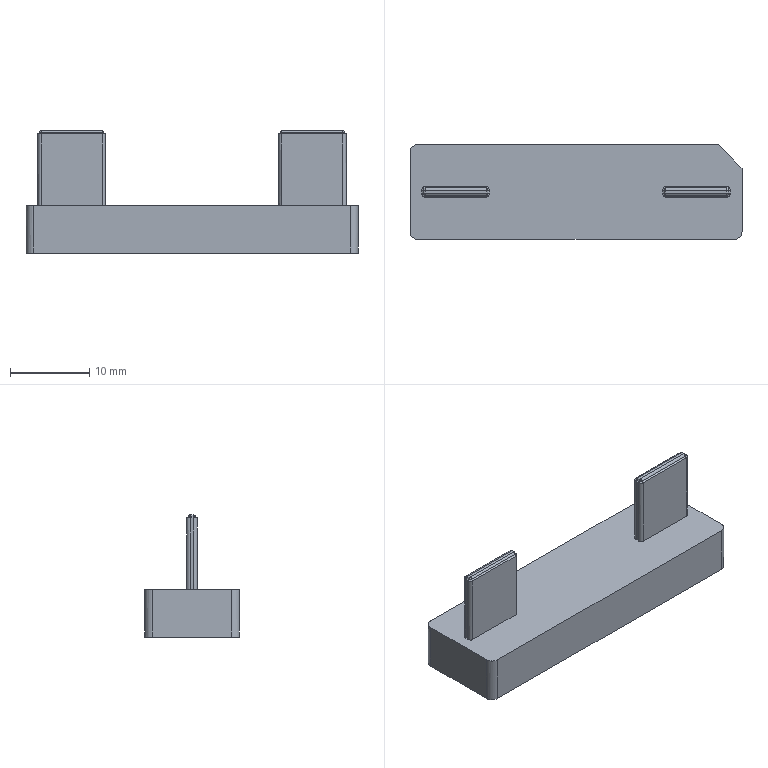NC program | PowerMill | posted with a generic post | part box 42 x 12 x 15.447 mm
Lines 1 to 1055 of 88764:
%
O0001
N104 ( POWERMILL CB  : 2026004.0)
N105 ( POST VER      : 2026.0.0.5161)
N106 ( OPTION FILE   : FANUC)
N107 ( OUTPUT WORKPLANE : WORLD)
N108 (  )
N109 ( TOOL LIST )
N110 (---------------------------------------)
N111 ( NO. | ID        | DIA.| TIP RAD|LENGTH)
N112 (---------------------------------------)
N113 (    1|D10C_1_1   |10.0 |  0.0   |70.88 )
N114 (    2|D4C_1_1    | 4.0 |  0.0   |64.64 )
N115 (    3|D10_1_1    |10.0 |  0.0   | 70.6 )
N116 (   14|D4_1_1     | 4.0 |  0.0   | 64.6 )
N117 (   13|TEXT_D4_1_1| 4.0 |  0.3   |64.72 )
N118 (---------------------------------------)
N119 (  )
N120 ( NUMBER OF TOOLPATHS: 10.0 )
N121 ( ESTIMATED PROGRAM DURATION: 0 HOURS 11 MIN 1 SEC)
N122 (  )
N123 G00 G21 G80 G40 G17
N124 G90
N125 G54
N126 G53 Z0.0
N127 (---------------)
N128 ( START TOOLPATH : 精公开粗01-扫面平行-D10C )
N129 (---------------)
N130 ( TOOL NO.    :1 )
N131 ( TOOL TYPE   : ENDMILL)
N132 ( TOOL ID     : D10C_1_1)
N133 ( TOOL DIA    : 10.0 LENGTH 70.88)
N134 T1
N135 M6
N136 S8000 M03
N137 G00 G90 X0.0 Y0.0
N138 G43 Z10.2 H1
N139
N140 G05 P10000 R4
N141 X28.78 Y8.78
N142 Z1.127
N143 G01 Z-0.073 F6000.0
N144 X23.78 F10000.0
N145 X-23.78
N146 Y2.9267
N147 X23.78
N148 Y-2.9267
N149 X-23.78
N150 Y-8.78
N151 X23.78
N152 X28.78
N153 G00 Z10.2
N154 G05 P0
N155 (---------------)
N156 ( END TOOLPATH : 精公开粗01-扫面平行-D10C )
N157 (---------------)
N158 ( START TOOLPATH : 精公开粗01-外形偏置-D10C )
N159 (---------------)
N160 G00 X0.0 Y0.0 Z9.877
N161 G05 P10000 R4
N162 X-32.559 Y-5.2036
N163 Z0.688
N164 G01 Z-0.512 F6000.0
N165 X-32.0315 F10000.0
N166 G03 X-27.284 Y-0.4561 I0.0 J4.7475
N167 G01 Y7.78
N168 G02 X-26.284 Y8.78 I1.0 J0.0
N169 G01 X26.284
N170 G02 X27.284 Y7.78 I0.0 J-1.0
N171 G01 Y0.8079
N172 X24.7331 Y0.7734
N173 X24.7496 Y-0.4555
N174 X24.7274 Y-0.7734
N175 X24.5895 Y-1.5469
N176 X24.3439 Y-2.3203
N177 X23.9729 Y-3.0937
N178 X23.4288 Y-3.8671
N179 X23.2028 Y-4.1175
N180 X22.6414 Y-4.6406
N181 X22.4294 Y-4.8022
N182 X21.6559 Y-5.2777
N183 X21.3815 Y-5.414
N184 X20.8825 Y-5.5978
N185 X20.1091 Y-5.796
N186 X19.3357 Y-5.8892
N187 X11.6014 Y-5.8877
N188 X10.828 Y-5.8639
N189 X10.0545 Y-5.7369
N190 X9.2811 Y-5.49
N191 X8.5077 Y-5.1105
N192 X7.8325 Y-4.6406
N193 X7.054 Y-3.8671
N194 X6.5022 Y-3.0937
N195 X6.1874 Y-2.453
N196 X5.8877 Y-1.5469
N197 X5.7582 Y-0.7734
N198 X5.7326 Y0.0
N199 X5.7455 Y0.7734
N200 X5.8745 Y1.5469
N201 X5.9581 Y1.8065
N202 X0.3867 Y2.4208
N203 G02 X0.0012 Y2.076 I-0.3848 J0.0424
N204 G01 X-0.0021
N205 X-0.0055 Y2.0761
N206 Y-2.2064
N207 G02 X0.3764 Y-2.5883 I0.0 J-0.3819
N208 G02 X-0.3874 I-0.3819 J0.0
N209 G02 X-0.0055 Y-2.2064 I0.3819 J0.0
N210 G01 Y2.0761
N211 G02 X-0.3628 Y2.5932 I0.0074 J0.3871
N212 G01 X-0.2934 Y2.788
N213 G02 X-0.0605 Y2.9519 I0.2324 J-0.0829
N214 G01 X0.0659 Y2.9517
N215 G02 X0.2982 Y2.787 I-0.0004 J-0.2468
N216 G01 X0.367 Y2.592
N217 X0.3865 Y2.5075
N218 X0.3867 Y2.4208
N219 X5.9581 Y1.8065
N220 X6.1874 Y2.5193
N221 X6.474 Y3.0937
N222 X6.9608 Y3.8106
N223 X7.7787 Y4.6406
N224 X8.5077 Y5.1518
N225 X8.9996 Y5.414
N226 X9.2811 Y5.534
N227 X10.0545 Y5.7837
N228 X10.828 Y5.9119
N229 X11.6014 Y5.9357
N230 X18.5622
N231 X19.3357 Y5.931
N232 X20.1091 Y5.8437
N233 X20.8825 Y5.6503
N234 X21.4813 Y5.414
N235 X22.4294 Y4.852
N236 X22.7051 Y4.6406
N237 X23.2028 Y4.1725
N238 X23.4735 Y3.8671
N239 X23.9762 Y3.1427
N240 X24.3653 Y2.3203
N241 X24.6064 Y1.5469
N242 X24.7331 Y0.7734
N243 X27.284 Y0.8079
N244 Y-7.78
N245 G02 X26.284 Y-8.78 I-1.0 J0.0
N246 G01 X-26.284
N247 G02 X-27.284 Y-7.78 I0.0 J1.0
N248 G01 Y-0.4561
N249 X-24.7496
N250 Y0.5704
N251 X-24.601 Y1.5469
N252 X-24.3658 Y2.3203
N253 X-23.9762 Y3.1313
N254 X-23.4728 Y3.8671
N255 X-23.2028 Y4.1739
N256 X-22.6998 Y4.6406
N257 X-22.4294 Y4.8544
N258 X-21.6559 Y5.3294
N259 X-20.8825 Y5.6492
N260 X-20.1091 Y5.8464
N261 X-19.3357 Y5.9311
N262 X-18.5622 Y5.9357
N263 X-11.6014 Y5.9359
N264 X-10.828 Y5.9134
N265 X-10.0545 Y5.7836
N266 X-9.2811 Y5.5312
N267 X-8.998 Y5.414
N268 X-8.5077 Y5.1537
N269 X-7.7744 Y4.6406
N270 X-7.007 Y3.8671
N271 X-6.476 Y3.0937
N272 X-6.1874 Y2.5182
N273 X-5.8693 Y1.5469
N274 X-5.7452 Y0.7734
N275 X-5.7326 Y0.0
N276 X-5.7584 Y-0.7734
N277 X-5.8875 Y-1.5469
N278 X-6.1289 Y-2.3203
N279 X-6.508 Y-3.0937
N280 X-6.9608 Y-3.7619
N281 X-7.7343 Y-4.5518
N282 X-8.5077 Y-5.1102
N283 X-9.104 Y-5.414
N284 X-10.0545 Y-5.7375
N285 X-10.828 Y-5.8615
N286 X-11.6014 Y-5.8877
N287 X-19.3357 Y-5.8895
N288 X-20.1091 Y-5.794
N289 X-20.8825 Y-5.5993
N290 X-21.3687 Y-5.414
N291 X-21.6559 Y-5.2777
N292 X-22.4294 Y-4.7988
N293 X-22.6434 Y-4.6406
N294 X-23.2028 Y-4.1175
N295 X-23.4283 Y-3.8671
N296 X-23.9762 Y-3.0927
N297 X-24.3515 Y-2.3203
N298 X-24.5954 Y-1.5469
N299 X-24.7275 Y-0.7734
N300 X-24.7496 Y-0.4561
N301 X-27.284
N302 G00 Z3.2989
N303 G01 X-32.559 Y-5.2036
N304 G00 Z0.2989
N305 G01 Z-0.9011 F6000.0
N306 X-32.0315 F10000.0
N307 G03 X-27.284 Y-0.4561 I0.0 J4.7475
N308 G01 Y-0.3163
N309 X-24.7764 Y-0.2095
N310 X-24.7854 Y0.0
N311 X-24.759 Y0.7734
N312 X-24.6351 Y1.5469
N313 X-24.398 Y2.3203
N314 X-24.0317 Y3.0937
N315 X-23.5026 Y3.8671
N316 X-23.2028 Y4.2075
N317 X-22.7401 Y4.6406
N318 X-22.4294 Y4.8821
N319 X-21.6559 Y5.3539
N320 X-20.8825 Y5.6732
N321 X-20.1091 Y5.8712
N322 X-19.3357 Y5.957
N323 X-18.5622 Y5.9622
N324 X-11.6014 Y5.9623
N325 X-10.828 Y5.9343
N326 X-10.0545 Y5.8051
N327 X-9.2811 Y5.5584
N328 X-8.9467 Y5.414
N329 X-8.5077 Y5.1812
N330 X-7.7402 Y4.6406
N331 X-6.9774 Y3.8671
N332 X-6.4482 Y3.0937
N333 X-6.0818 Y2.3203
N334 X-5.8449 Y1.5469
N335 X-5.721 Y0.7734
N336 X-5.6946 Y0.0
N337 X-5.7236 Y-0.7734
N338 X-5.852 Y-1.5469
N339 X-6.0943 Y-2.3203
N340 X-6.4664 Y-3.0937
N341 X-6.9608 Y-3.8149
N342 X-7.7343 Y-4.6004
N343 X-8.5077 Y-5.1489
N344 X-9.016 Y-5.414
N345 X-9.2811 Y-5.5261
N346 X-10.0545 Y-5.773
N347 X-10.828 Y-5.9012
N348 X-11.6014 Y-5.93
N349 X-18.5622
N350 X-19.3357 Y-5.925
N351 X-20.1091 Y-5.837
N352 X-20.8825 Y-5.6427
N353 X-21.6559 Y-5.3218
N354 X-22.4294 Y-4.8484
N355 X-22.6992 Y-4.6406
N356 X-23.2028 Y-4.1755
N357 X-23.4766 Y-3.8671
N358 X-23.9762 Y-3.1574
N359 X-24.3861 Y-2.3203
N360 X-24.6279 Y-1.5469
N361 X-24.7496 Y-0.8378
N362 X-24.7764 Y-0.2095
N363 X-27.284 Y-0.3163
N364 Y7.78
N365 G02 X-26.284 Y8.78 I1.0 J0.0
N366 G01 X26.284
N367 G02 X27.284 Y7.78 I0.0 J-1.0
N368 G01 Y0.3202
N369 X24.7764 Y0.2171
N370 X24.7854 Y0.0
N371 X24.7564 Y-0.7734
N372 X24.628 Y-1.5469
N373 X24.3857 Y-2.3203
N374 X24.0136 Y-3.0937
N375 X23.4763 Y-3.8671
N376 X23.2028 Y-4.1755
N377 X22.6976 Y-4.6406
N378 X22.4294 Y-4.85
N379 X21.6559 Y-5.3218
N380 X21.4641 Y-5.414
N381 X20.8825 Y-5.641
N382 X20.1091 Y-5.839
N383 X19.3357 Y-5.9248
N384 X18.5622 Y-5.93
N385 X11.6014
N386 X10.828 Y-5.903
N387 X10.0545 Y-5.7722
N388 X9.2811 Y-5.5263
N389 X9.0159 Y-5.414
N390 X8.5077 Y-5.1494
N391 X7.7808 Y-4.6406
N392 X7.0034 Y-3.8671
N393 X6.4666 Y-3.0937
N394 X6.0939 Y-2.3203
N395 X5.852 Y-1.5469
N396 X5.7236 Y-0.7734
N397 X5.6946 Y0.0
N398 X5.7209 Y0.7734
N399 X5.8449 Y1.5469
N400 X6.082 Y2.3203
N401 X6.4483 Y3.0937
N402 X6.9773 Y3.8671
N403 X7.7343 Y4.6359
N404 X8.5077 Y5.1809
N405 X8.9467 Y5.414
N406 X9.2811 Y5.5584
N407 X10.0545 Y5.8053
N408 X10.828 Y5.9334
N409 X11.6014 Y5.9622
N410 X18.5622
N411 X19.3357 Y5.9573
N412 X20.1091 Y5.8705
N413 X20.8825 Y5.6742
N414 X21.5333 Y5.414
N415 X22.4294 Y4.8799
N416 X22.7397 Y4.6406
N417 X23.2028 Y4.2056
N418 X23.5026 Y3.8671
N419 X23.9762 Y3.1891
N420 X24.3982 Y2.3203
N421 X24.635 Y1.5469
N422 X24.7496 Y0.8683
N423 X24.7764 Y0.2171
N424 X27.284 Y0.3202
N425 Y-7.78
N426 G02 X26.284 Y-8.78 I-1.0 J0.0
N427 G01 X-0.0002
N428 Y-4.28
N429 X-1.312
N430 G02 X-1.7891 Y-3.6305 I0.0 J0.5
N431 G01 X-1.5578 Y-2.8921
N432 X-1.4748 Y-2.5906
N433 X-1.4128 Y-2.2841
N434 X-1.2844 Y-1.5107
N435 X-1.2465 Y-1.2273
N436 X-1.2267 Y-0.942
N437 X-1.1977 Y-0.1686
N438 X-1.1946 Y-0.0075
N439 X-1.1972 Y0.1537
N440 X-1.2236 Y0.9271
N441 X-1.242 Y1.2071
N442 X-1.2777 Y1.4853
N443 X-1.4016 Y2.2587
N444 X-1.4614 Y2.5642
N445 X-1.5423 Y2.8649
N446 X-1.7777 Y3.6336
N447 G02 X-1.2997 Y4.28 I0.478 J0.1464
N448 G01 X1.2999
N449 G02 X1.7779 Y3.6335 I0.0 J-0.5
N450 G01 X1.5426 Y2.8658
N451 X1.4616 Y2.565
N452 X1.4017 Y2.2594
N453 X1.2777 Y1.486
N454 X1.2419 Y1.2071
N455 X1.2235 Y0.9266
N456 X1.1972 Y0.1531
N457 X1.1946 Y-0.0077
N458 X1.1977 Y-0.1686
N459 X1.2267 Y-0.942
N460 X1.2465 Y-1.2272
N461 X1.2844 Y-1.5106
N462 X1.4128 Y-2.284
N463 X1.4745 Y-2.5896
N464 X1.5572 Y-2.8901
N465 X1.7888 Y-3.6307
N466 G02 X1.3116 Y-4.28 I-0.4772 J-0.1493
N467 G01 X-0.0002
N468 Y-8.78
N469 X-26.284
N470 G02 X-27.284 Y-7.78 I0.0 J1.0
N471 G01 Y-0.4561
N472 G00 Z2.9099
N473 G01 X-32.559 Y-5.2036
N474 G00 Z-0.0901
N475 G01 Z-1.2901 F6000.0
N476 X-32.0315 F10000.0
N477 G03 X-27.284 Y-0.4561 I0.0 J4.7475
N478 G01 Y-0.3164
N479 X-24.7764 Y-0.2095
N480 X-24.7854 Y0.0
N481 X-24.759 Y0.7734
N482 X-24.6351 Y1.5469
N483 X-24.398 Y2.3203
N484 X-24.0317 Y3.0937
N485 X-23.5026 Y3.8671
N486 X-23.2028 Y4.2075
N487 X-22.7401 Y4.6406
N488 X-22.4294 Y4.8821
N489 X-21.6559 Y5.3539
N490 X-20.8825 Y5.6732
N491 X-20.1091 Y5.8712
N492 X-19.3357 Y5.957
N493 X-18.5622 Y5.9622
N494 X-11.6014 Y5.9623
N495 X-10.828 Y5.9343
N496 X-10.0545 Y5.8051
N497 X-9.2811 Y5.5584
N498 X-8.9467 Y5.414
N499 X-8.5077 Y5.1812
N500 X-7.7402 Y4.6406
N501 X-6.9774 Y3.8671
N502 X-6.4482 Y3.0937
N503 X-6.0818 Y2.3203
N504 X-5.8449 Y1.5469
N505 X-5.721 Y0.7734
N506 X-5.6946 Y0.0
N507 X-5.7236 Y-0.7734
N508 X-5.852 Y-1.5469
N509 X-6.0943 Y-2.3203
N510 X-6.4664 Y-3.0937
N511 X-6.9608 Y-3.8149
N512 X-7.7343 Y-4.6004
N513 X-8.5077 Y-5.1489
N514 X-9.016 Y-5.414
N515 X-9.2811 Y-5.5262
N516 X-10.0545 Y-5.773
N517 X-10.828 Y-5.9012
N518 X-11.6014 Y-5.93
N519 X-18.5622
N520 X-19.3357 Y-5.925
N521 X-20.1091 Y-5.837
N522 X-20.8825 Y-5.6427
N523 X-21.6559 Y-5.3218
N524 X-22.4294 Y-4.8484
N525 X-22.6992 Y-4.6406
N526 X-23.2028 Y-4.1755
N527 X-23.4766 Y-3.8671
N528 X-23.9762 Y-3.1574
N529 X-24.3861 Y-2.3203
N530 X-24.6279 Y-1.5469
N531 X-24.7496 Y-0.8378
N532 X-24.7764 Y-0.2095
N533 X-27.284 Y-0.3164
N534 Y7.78
N535 G02 X-26.284 Y8.78 I1.0 J0.0
N536 G01 X26.284
N537 G02 X27.284 Y7.78 I0.0 J-1.0
N538 G01 Y0.3202
N539 X24.7764 Y0.2171
N540 X24.7854 Y0.0
N541 X24.7564 Y-0.7734
N542 X24.628 Y-1.5469
N543 X24.3857 Y-2.3203
N544 X24.0136 Y-3.0937
N545 X23.4763 Y-3.8671
N546 X23.2028 Y-4.1756
N547 X22.6976 Y-4.6406
N548 X22.4294 Y-4.85
N549 X21.6559 Y-5.3218
N550 X21.4641 Y-5.414
N551 X20.8825 Y-5.641
N552 X20.1091 Y-5.839
N553 X19.3357 Y-5.9248
N554 X18.5622 Y-5.93
N555 X11.6014
N556 X10.828 Y-5.903
N557 X10.0545 Y-5.7722
N558 X9.2811 Y-5.5263
N559 X9.0159 Y-5.414
N560 X8.5077 Y-5.1494
N561 X7.7808 Y-4.6406
N562 X7.0034 Y-3.8671
N563 X6.4666 Y-3.0937
N564 X6.0939 Y-2.3203
N565 X5.852 Y-1.5469
N566 X5.7236 Y-0.7734
N567 X5.6946 Y0.0
N568 X5.7209 Y0.7734
N569 X5.8449 Y1.5469
N570 X6.082 Y2.3203
N571 X6.4483 Y3.0937
N572 X6.9773 Y3.8671
N573 X7.7343 Y4.6359
N574 X8.5077 Y5.1809
N575 X8.9466 Y5.414
N576 X9.2811 Y5.5584
N577 X10.0545 Y5.8053
N578 X10.828 Y5.9334
N579 X11.6014 Y5.9623
N580 X18.5622 Y5.9622
N581 X19.3357 Y5.9573
N582 X20.1091 Y5.8705
N583 X20.8825 Y5.6742
N584 X21.5333 Y5.414
N585 X22.4294 Y4.8799
N586 X22.7397 Y4.6406
N587 X23.2028 Y4.2056
N588 X23.5026 Y3.8671
N589 X23.9762 Y3.1891
N590 X24.3982 Y2.3203
N591 X24.6351 Y1.5469
N592 X24.7496 Y0.8683
N593 X24.7764 Y0.2171
N594 X27.284 Y0.3202
N595 Y-7.78
N596 G02 X26.284 Y-8.78 I-1.0 J0.0
N597 G01 X-0.0002
N598 Y-4.28
N599 X-1.312
N600 G02 X-1.7891 Y-3.6305 I0.0 J0.5
N601 G01 X-1.5578 Y-2.8921
N602 X-1.4747 Y-2.5906
N603 X-1.4128 Y-2.2841
N604 X-1.2844 Y-1.5107
N605 X-1.2465 Y-1.2273
N606 X-1.2267 Y-0.942
N607 X-1.1977 Y-0.1686
N608 X-1.1946 Y-0.0075
N609 X-1.1972 Y0.1537
N610 X-1.2236 Y0.9271
N611 X-1.2419 Y1.2071
N612 X-1.2777 Y1.4853
N613 X-1.4016 Y2.2587
N614 X-1.4614 Y2.5642
N615 X-1.5423 Y2.8649
N616 X-1.7777 Y3.6336
N617 G02 X-1.2997 Y4.28 I0.478 J0.1464
N618 G01 X1.2999
N619 G02 X1.7779 Y3.6335 I0.0 J-0.5
N620 G01 X1.5426 Y2.8658
N621 X1.4616 Y2.565
N622 X1.4017 Y2.2594
N623 X1.2777 Y1.486
N624 X1.2419 Y1.2071
N625 X1.2235 Y0.9266
N626 X1.1972 Y0.1531
N627 X1.1946 Y-0.0077
N628 X1.1977 Y-0.1686
N629 X1.2267 Y-0.942
N630 X1.2465 Y-1.2272
N631 X1.2844 Y-1.5106
N632 X1.4128 Y-2.284
N633 X1.4745 Y-2.5896
N634 X1.5572 Y-2.8901
N635 X1.7888 Y-3.6307
N636 G02 X1.3116 Y-4.28 I-0.4772 J-0.1493
N637 G01 X-0.0002
N638 Y-8.78
N639 X-26.284
N640 G02 X-27.284 Y-7.78 I0.0 J1.0
N641 G01 Y-0.4561
N642 G00 Z2.5208
N643 G01 X-32.559 Y-5.2036
N644 G00 Z-0.4792
N645 G01 Z-1.6792 F6000.0
N646 X-32.0315 F10000.0
N647 G03 X-27.284 Y-0.4561 I0.0 J4.7475
N648 G01 Y-0.3164
N649 X-24.7764 Y-0.2095
N650 X-24.7854 Y0.0
N651 X-24.759 Y0.7734
N652 X-24.6351 Y1.5469
N653 X-24.398 Y2.3203
N654 X-24.0317 Y3.0937
N655 X-23.5026 Y3.8671
N656 X-23.2028 Y4.2075
N657 X-22.7401 Y4.6406
N658 X-22.4294 Y4.8821
N659 X-21.6559 Y5.3539
N660 X-20.8825 Y5.6732
N661 X-20.1091 Y5.8712
N662 X-19.3357 Y5.957
N663 X-18.5622 Y5.9622
N664 X-11.6014 Y5.9623
N665 X-10.828 Y5.9343
N666 X-10.0545 Y5.8051
N667 X-9.2811 Y5.5584
N668 X-8.9467 Y5.414
N669 X-8.5077 Y5.1812
N670 X-7.7402 Y4.6406
N671 X-6.9774 Y3.8671
N672 X-6.4482 Y3.0937
N673 X-6.0818 Y2.3203
N674 X-5.8449 Y1.5469
N675 X-5.721 Y0.7734
N676 X-5.6946 Y0.0
N677 X-5.7236 Y-0.7734
N678 X-5.852 Y-1.5469
N679 X-6.0943 Y-2.3203
N680 X-6.4664 Y-3.0937
N681 X-6.9608 Y-3.8149
N682 X-7.7343 Y-4.6004
N683 X-8.5077 Y-5.1489
N684 X-9.0159 Y-5.414
N685 X-9.2811 Y-5.5262
N686 X-10.0545 Y-5.7731
N687 X-10.828 Y-5.9012
N688 X-11.6014 Y-5.93
N689 X-18.5622
N690 X-19.3357 Y-5.925
N691 X-20.1091 Y-5.837
N692 X-20.8825 Y-5.6427
N693 X-21.6559 Y-5.3218
N694 X-22.4294 Y-4.8484
N695 X-22.6992 Y-4.6406
N696 X-23.2028 Y-4.1755
N697 X-23.4766 Y-3.8671
N698 X-23.9762 Y-3.1574
N699 X-24.3861 Y-2.3203
N700 X-24.6279 Y-1.5469
N701 X-24.7496 Y-0.8378
N702 X-24.7764 Y-0.2095
N703 X-27.284 Y-0.3164
N704 Y7.78
N705 G02 X-26.284 Y8.78 I1.0 J0.0
N706 G01 X26.284
N707 G02 X27.284 Y7.78 I0.0 J-1.0
N708 G01 Y0.3202
N709 X24.7764 Y0.2171
N710 X24.7854 Y0.0
N711 X24.7564 Y-0.7734
N712 X24.628 Y-1.5469
N713 X24.3857 Y-2.3203
N714 X24.0136 Y-3.0937
N715 X23.4763 Y-3.8671
N716 X23.2028 Y-4.1756
N717 X22.6976 Y-4.6406
N718 X22.4294 Y-4.85
N719 X21.6559 Y-5.3218
N720 X21.4641 Y-5.414
N721 X20.8825 Y-5.641
N722 X20.1091 Y-5.839
N723 X19.3357 Y-5.9248
N724 X18.5622 Y-5.93
N725 X11.6014
N726 X10.828 Y-5.903
N727 X10.0545 Y-5.7722
N728 X9.2811 Y-5.5263
N729 X9.0159 Y-5.414
N730 X8.5077 Y-5.1494
N731 X7.7808 Y-4.6406
N732 X7.0034 Y-3.8671
N733 X6.4666 Y-3.0937
N734 X6.0939 Y-2.3203
N735 X5.852 Y-1.5469
N736 X5.7236 Y-0.7734
N737 X5.6946 Y0.0
N738 X5.7209 Y0.7734
N739 X5.8449 Y1.5469
N740 X6.082 Y2.3203
N741 X6.4483 Y3.0937
N742 X6.9773 Y3.8671
N743 X7.7343 Y4.6359
N744 X8.5077 Y5.1809
N745 X8.9466 Y5.414
N746 X9.2811 Y5.5585
N747 X10.0545 Y5.8053
N748 X10.828 Y5.9334
N749 X11.6014 Y5.9623
N750 X18.5622 Y5.9622
N751 X19.3357 Y5.9573
N752 X20.1091 Y5.8705
N753 X20.8825 Y5.6742
N754 X21.5333 Y5.414
N755 X22.4294 Y4.8799
N756 X22.7397 Y4.6406
N757 X23.2028 Y4.2056
N758 X23.5026 Y3.8671
N759 X23.9762 Y3.1892
N760 X24.3982 Y2.3203
N761 X24.6351 Y1.5469
N762 X24.7496 Y0.8683
N763 X24.7764 Y0.2171
N764 X27.284 Y0.3202
N765 Y-7.78
N766 G02 X26.284 Y-8.78 I-1.0 J0.0
N767 G01 X-0.0002
N768 Y-4.28
N769 X-1.312
N770 G02 X-1.7891 Y-3.6305 I0.0 J0.5
N771 G01 X-1.5578 Y-2.8921
N772 X-1.4747 Y-2.5906
N773 X-1.4128 Y-2.2841
N774 X-1.2844 Y-1.5107
N775 X-1.2465 Y-1.2273
N776 X-1.2267 Y-0.942
N777 X-1.1977 Y-0.1686
N778 X-1.1946 Y-0.0075
N779 X-1.1972 Y0.1537
N780 X-1.2236 Y0.9271
N781 X-1.2419 Y1.2071
N782 X-1.2777 Y1.4853
N783 X-1.4016 Y2.2587
N784 X-1.4614 Y2.5642
N785 X-1.5423 Y2.8649
N786 X-1.7777 Y3.6336
N787 G02 X-1.2997 Y4.28 I0.478 J0.1464
N788 G01 X1.2999
N789 G02 X1.7779 Y3.6335 I-0.0001 J-0.5
N790 G01 X1.5426 Y2.8658
N791 X1.4616 Y2.565
N792 X1.4017 Y2.2594
N793 X1.2777 Y1.486
N794 X1.2419 Y1.2071
N795 X1.2235 Y0.9266
N796 X1.1972 Y0.1531
N797 X1.1946 Y-0.0077
N798 X1.1977 Y-0.1686
N799 X1.2267 Y-0.942
N800 X1.2465 Y-1.2272
N801 X1.2844 Y-1.5106
N802 X1.4128 Y-2.284
N803 X1.4745 Y-2.5896
N804 X1.5572 Y-2.8901
N805 X1.7888 Y-3.6307
N806 G02 X1.3116 Y-4.28 I-0.4772 J-0.1493
N807 G01 X-0.0002
N808 Y-8.78
N809 X-26.284
N810 G02 X-27.284 Y-7.78 I0.0 J1.0
N811 G01 Y-0.4561
N812 G00 Z2.1318
N813 G01 X-32.559 Y-5.2036
N814 G00 Z-0.8682
N815 G01 Z-2.0682 F6000.0
N816 X-32.0315 F10000.0
N817 G03 X-27.284 Y-0.4561 I0.0 J4.7475
N818 G01 Y-0.3164
N819 X-24.7764 Y-0.2095
N820 X-24.7854 Y0.0
N821 X-24.759 Y0.7734
N822 X-24.6351 Y1.5469
N823 X-24.398 Y2.3203
N824 X-24.0318 Y3.0937
N825 X-23.5026 Y3.8671
N826 X-23.2028 Y4.2075
N827 X-22.7401 Y4.6406
N828 X-22.4294 Y4.8821
N829 X-21.6559 Y5.354
N830 X-20.8825 Y5.6732
N831 X-20.1091 Y5.8712
N832 X-19.3357 Y5.9571
N833 X-18.5622 Y5.9622
N834 X-11.6014 Y5.9623
N835 X-10.828 Y5.9343
N836 X-10.0545 Y5.8051
N837 X-9.2811 Y5.5585
N838 X-8.9467 Y5.414
N839 X-8.5077 Y5.1812
N840 X-7.7402 Y4.6406
N841 X-6.9774 Y3.8671
N842 X-6.4482 Y3.0937
N843 X-6.0818 Y2.3203
N844 X-5.8449 Y1.5469
N845 X-5.721 Y0.7734
N846 X-5.6946 Y0.0
N847 X-5.7236 Y-0.7734
N848 X-5.852 Y-1.5469
N849 X-6.0943 Y-2.3203
N850 X-6.4664 Y-3.0937
N851 X-6.9608 Y-3.8149
N852 X-7.7343 Y-4.6004
N853 X-8.5077 Y-5.1489
N854 X-9.0159 Y-5.414
N855 X-9.2811 Y-5.5262
N856 X-10.0545 Y-5.7731
N857 X-10.828 Y-5.9012
N858 X-11.6014 Y-5.93
N859 X-18.5622
N860 X-19.3357 Y-5.925
N861 X-20.1091 Y-5.837
N862 X-20.8825 Y-5.6427
N863 X-21.6559 Y-5.3218
N864 X-22.4294 Y-4.8484
N865 X-22.6992 Y-4.6406
N866 X-23.2028 Y-4.1755
N867 X-23.4766 Y-3.8671
N868 X-23.9762 Y-3.1574
N869 X-24.3861 Y-2.3203
N870 X-24.6279 Y-1.5469
N871 X-24.7496 Y-0.8378
N872 X-24.7764 Y-0.2095
N873 X-27.284 Y-0.3164
N874 Y7.78
N875 G02 X-26.284 Y8.78 I1.0 J0.0
N876 G01 X26.284
N877 G02 X27.284 Y7.78 I0.0 J-1.0
N878 G01 Y0.3202
N879 X24.7764 Y0.2171
N880 X24.7854 Y0.0
N881 X24.7564 Y-0.7734
N882 X24.628 Y-1.5469
N883 X24.3857 Y-2.3203
N884 X24.0136 Y-3.0937
N885 X23.4763 Y-3.8671
N886 X23.2028 Y-4.1756
N887 X22.6976 Y-4.6406
N888 X22.4294 Y-4.85
N889 X21.6559 Y-5.3218
N890 X21.4641 Y-5.414
N891 X20.8825 Y-5.641
N892 X20.1091 Y-5.839
N893 X19.3357 Y-5.9248
N894 X18.5622 Y-5.93
N895 X11.6014
N896 X10.828 Y-5.903
N897 X10.0545 Y-5.7722
N898 X9.2811 Y-5.5263
N899 X9.0159 Y-5.414
N900 X8.5077 Y-5.1494
N901 X7.7808 Y-4.6406
N902 X7.0034 Y-3.8671
N903 X6.4666 Y-3.0937
N904 X6.0939 Y-2.3203
N905 X5.852 Y-1.5469
N906 X5.7236 Y-0.7734
N907 X5.6946 Y0.0
N908 X5.7209 Y0.7734
N909 X5.8449 Y1.5469
N910 X6.082 Y2.3203
N911 X6.4483 Y3.0937
N912 X6.9773 Y3.8671
N913 X7.7343 Y4.6359
N914 X8.5077 Y5.181
N915 X8.9466 Y5.414
N916 X9.2811 Y5.5585
N917 X10.0545 Y5.8053
N918 X10.828 Y5.9334
N919 X11.6014 Y5.9623
N920 X18.5622 Y5.9622
N921 X19.3357 Y5.9573
N922 X20.1091 Y5.8705
N923 X20.8825 Y5.6742
N924 X21.5334 Y5.414
N925 X22.4294 Y4.8799
N926 X22.7398 Y4.6406
N927 X23.2028 Y4.2056
N928 X23.5026 Y3.8671
N929 X23.9762 Y3.1892
N930 X24.3982 Y2.3203
N931 X24.6351 Y1.5469
N932 X24.7496 Y0.8683
N933 X24.7764 Y0.2171
N934 X27.284 Y0.3202
N935 Y-7.78
N936 G02 X26.284 Y-8.78 I-1.0 J0.0
N937 G01 X-0.0002
N938 Y-4.28
N939 X-1.312
N940 G02 X-1.7891 Y-3.6305 I0.0 J0.5
N941 G01 X-1.5578 Y-2.8921
N942 X-1.4747 Y-2.5906
N943 X-1.4128 Y-2.2841
N944 X-1.2844 Y-1.5106
N945 X-1.2465 Y-1.2272
N946 X-1.2267 Y-0.942
N947 X-1.1977 Y-0.1686
N948 X-1.1946 Y-0.0075
N949 X-1.1972 Y0.1537
N950 X-1.2236 Y0.9271
N951 X-1.2419 Y1.2071
N952 X-1.2777 Y1.4853
N953 X-1.4016 Y2.2587
N954 X-1.4614 Y2.5642
N955 X-1.5423 Y2.8649
N956 X-1.7777 Y3.6336
N957 G02 X-1.2997 Y4.28 I0.478 J0.1464
N958 G01 X1.2998
N959 G02 X1.7779 Y3.6335 I0.0 J-0.5
N960 G01 X1.5425 Y2.8658
N961 X1.4616 Y2.565
N962 X1.4017 Y2.2594
N963 X1.2777 Y1.486
N964 X1.2418 Y1.2071
N965 X1.2235 Y0.9266
N966 X1.1972 Y0.1531
N967 X1.1946 Y-0.0077
N968 X1.1977 Y-0.1686
N969 X1.2267 Y-0.942
N970 X1.2465 Y-1.2272
N971 X1.2844 Y-1.5106
N972 X1.4128 Y-2.284
N973 X1.4745 Y-2.5896
N974 X1.5572 Y-2.8901
N975 X1.7888 Y-3.6307
N976 G02 X1.3116 Y-4.28 I-0.4772 J-0.1493
N977 G01 X-0.0002
N978 Y-8.78
N979 X-26.284
N980 G02 X-27.284 Y-7.78 I0.0 J1.0
N981 G01 Y-0.4561
N982 G00 Z1.7427
N983 G01 X-32.559 Y-5.2036
N984 G00 Z-1.2573
N985 G01 Z-2.4573 F6000.0
N986 X-32.0315 F10000.0
N987 G03 X-27.284 Y-0.4561 I0.0 J4.7475
N988 G01 Y-0.3164
N989 X-24.7764 Y-0.2095
N990 X-24.7854 Y0.0
N991 X-24.759 Y0.7734
N992 X-24.6351 Y1.5469
N993 X-24.398 Y2.3203
N994 X-24.0318 Y3.0937
N995 X-23.5026 Y3.8671
N996 X-23.2028 Y4.2075
N997 X-22.7401 Y4.6406
N998 X-22.4294 Y4.8822
N999 X-21.6559 Y5.354
N1000 X-20.8825 Y5.6732
N1001 X-20.1091 Y5.8712
N1002 X-19.3357 Y5.9571
N1003 X-18.5622 Y5.9623
N1004 X-11.6014
N1005 X-10.828 Y5.9343
N1006 X-10.0545 Y5.8051
N1007 X-9.2811 Y5.5585
N1008 X-8.9466 Y5.414
N1009 X-8.5077 Y5.1812
N1010 X-7.7402 Y4.6406
N1011 X-6.9773 Y3.8671
N1012 X-6.4482 Y3.0937
N1013 X-6.0818 Y2.3203
N1014 X-5.8449 Y1.5469
N1015 X-5.721 Y0.7734
N1016 X-5.6946 Y0.0
N1017 X-5.7236 Y-0.7734
N1018 X-5.852 Y-1.5469
N1019 X-6.0943 Y-2.3203
N1020 X-6.4664 Y-3.0937
N1021 X-6.9608 Y-3.8149
N1022 X-7.7343 Y-4.6004
N1023 X-8.5077 Y-5.1489
N1024 X-9.0159 Y-5.414
N1025 X-9.2811 Y-5.5262
N1026 X-10.0545 Y-5.7731
N1027 X-10.828 Y-5.9012
N1028 X-11.6014 Y-5.93
N1029 X-18.5622
N1030 X-19.3357 Y-5.925
N1031 X-20.1091 Y-5.837
N1032 X-20.8825 Y-5.6427
N1033 X-21.6559 Y-5.3218
N1034 X-22.4294 Y-4.8484
N1035 X-22.6992 Y-4.6406
N1036 X-23.2028 Y-4.1755
N1037 X-23.4766 Y-3.8671
N1038 X-23.9762 Y-3.1574
N1039 X-24.3861 Y-2.3203
N1040 X-24.6279 Y-1.5469
N1041 X-24.7496 Y-0.8378
N1042 X-24.7764 Y-0.2095
N1043 X-27.284 Y-0.3164
N1044 Y7.78
N1045 G02 X-26.284 Y8.78 I1.0 J0.0
N1046 G01 X26.284
N1047 G02 X27.284 Y7.78 I0.0 J-1.0
N1048 G01 Y0.3203
N1049 X24.7764 Y0.2171
N1050 X24.7854 Y0.0
N1051 X24.7564 Y-0.7734
N1052 X24.628 Y-1.5469
N1053 X24.3857 Y-2.3203
N1054 X24.0136 Y-3.0937
N1055 X23.4764 Y-3.8671
N1056 X23.2028 Y-4.1756
N1057 X22.6976 Y-4.6406
N1058 X22.4294 Y-4.85
N1059 X21.6559 Y-5.3218
N1060 X21.4641 Y-5.414
N1061 X20.8825 Y-5.641
N1062 X20.1091 Y-5.839
N1063 X19.3357 Y-5.9248
N1064 X18.5622 Y-5.93
N1065 X11.6014
N1066 X10.828 Y-5.903
N1067 X10.0545 Y-5.7722
N1068 X9.2811 Y-5.5263
N1069 X9.0159 Y-5.414
N1070 X8.5077 Y-5.1494
N1071 X7.7808 Y-4.6406
N1072 X7.0034 Y-3.8671
N1073 X6.4666 Y-3.0937
N1074 X6.0939 Y-2.3203
N1075 X5.852 Y-1.5469
N1076 X5.7236 Y-0.7734
N1077 X5.6946 Y0.0
N1078 X5.7209 Y0.7734
N1079 X5.8449 Y1.5469
N1080 X6.082 Y2.3203
N1081 X6.4483 Y3.0937
N1082 X6.9773 Y3.8671
N1083 X7.7343 Y4.6359
N1084 X8.5077 Y5.181
N1085 X8.9466 Y5.414
N1086 X9.2811 Y5.5585
N1087 X10.0545 Y5.8053
N1088 X10.828 Y5.9334
N1089 X11.6014 Y5.9623
N1090 X18.5622
N1091 X19.3357 Y5.9573
N1092 X20.1091 Y5.8705
N1093 X20.8825 Y5.6743
N1094 X21.5334 Y5.414
N1095 X22.4294 Y4.8799
N1096 X22.7398 Y4.6406
N1097 X23.2028 Y4.2056
N1098 X23.5026 Y3.8671
N1099 X23.9762 Y3.1892
N1100 X24.3982 Y2.3203
N1101 X24.6351 Y1.5469
N1102 X24.7496 Y0.8683
N1103 X24.7764 Y0.2171
N1104 X27.284 Y0.3203
N1105 Y-7.78
N1106 G02 X26.284 Y-8.78 I-1.0 J0.0
N1107 G01 X-0.0002
N1108 Y-4.28
N1109 X-1.312
N1110 G02 X-1.7891 Y-3.6305 I0.0 J0.5
N1111 G01 X-1.5578 Y-2.8921
N1112 X-1.4747 Y-2.5906
N1113 X-1.4128 Y-2.2841
N1114 X-1.2844 Y-1.5106
N1115 X-1.2465 Y-1.2272
N1116 X-1.2267 Y-0.942
N1117 X-1.1977 Y-0.1686
N1118 X-1.1946 Y-0.0075
N1119 X-1.1972 Y0.1537
N1120 X-1.2236 Y0.9271
N1121 X-1.2419 Y1.2071
N1122 X-1.2777 Y1.4853
N1123 X-1.4016 Y2.2588
N1124 X-1.4614 Y2.5642
N1125 X-1.5423 Y2.8649
N1126 X-1.7777 Y3.6336
N1127 G02 X-1.2997 Y4.28 I0.478 J0.1464
N1128 G01 X1.2998
N1129 G02 X1.7779 Y3.6335 I0.0 J-0.5
N1130 G01 X1.5425 Y2.8658
N1131 X1.4616 Y2.565
N1132 X1.4017 Y2.2594
N1133 X1.2777 Y1.486
N1134 X1.2418 Y1.2071
N1135 X1.2235 Y0.9266
N1136 X1.1972 Y0.1531
N1137 X1.1946 Y-0.0077
N1138 X1.1977 Y-0.1686
N1139 X1.2267 Y-0.942
N1140 X1.2465 Y-1.2272
N1141 X1.2843 Y-1.5106
N1142 X1.4128 Y-2.284
N1143 X1.4745 Y-2.5896
N1144 X1.5571 Y-2.8901
N1145 X1.7888 Y-3.6307
N1146 G02 X1.3116 Y-4.28 I-0.4772 J-0.1493
N1147 G01 X-0.0002
N1148 Y-8.78
N1149 X-26.284
N1150 G02 X-27.284 Y-7.78 I0.0 J1.0
N1151 G01 Y-0.4561
N1152 G00 Z1.3537